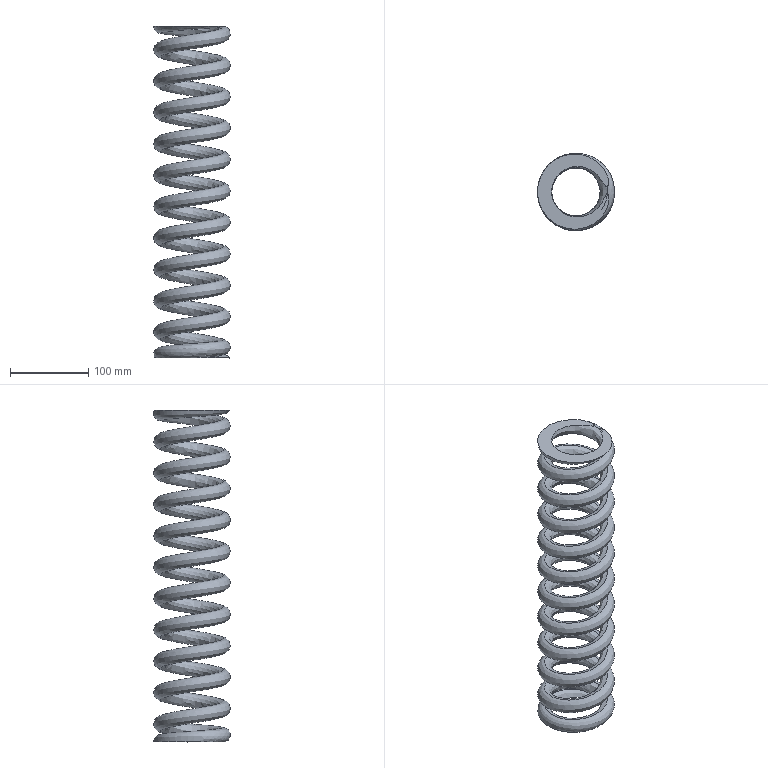Part | SolidWorks | features Helix 1, ICE 1, RefAxis 1, Sweep 1 | 1 solid | 5 faces | box 98 x 98 x 423 mm | volume 719372 mm3 | plane 3 | spline 2